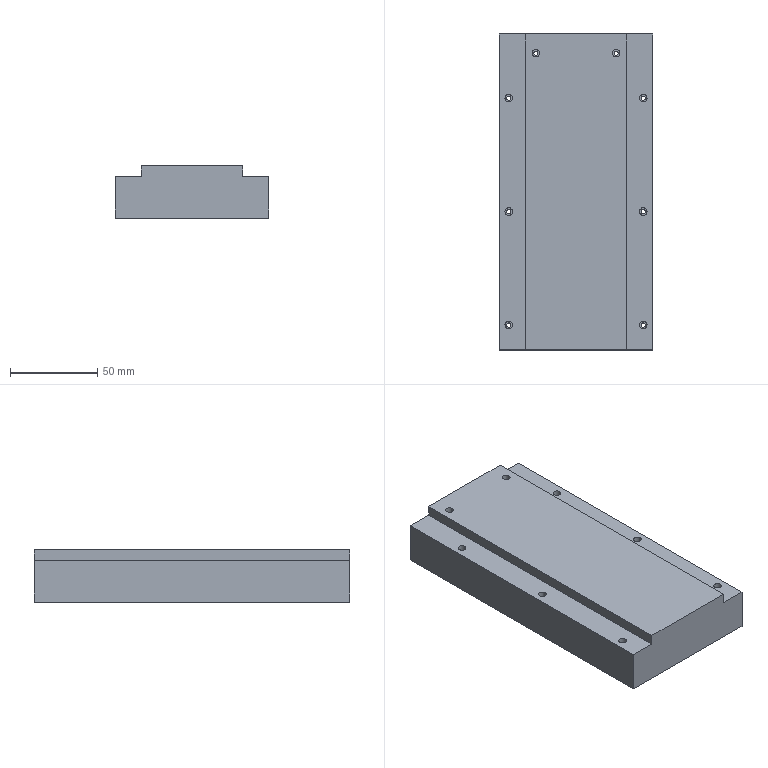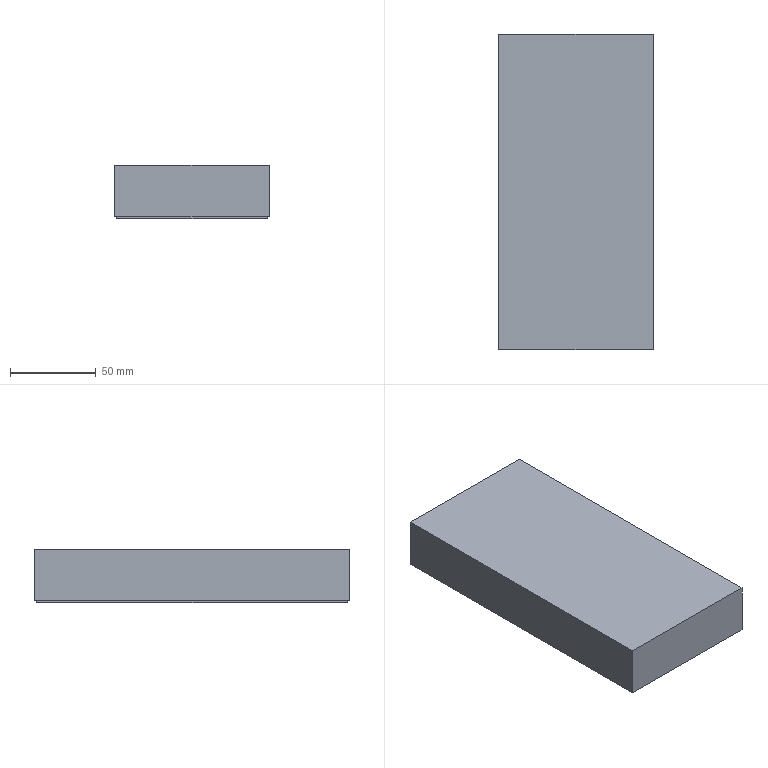CAM job | NX | 3+2 milling, drilling | part box 88 x 181.05 x 30 mm | stock box 90 x 184 x 31 mm
Tools:
number,name,description,diameter,corner_radius,flute_length,length,flutes
0,D4.2,Milling Tool-5 Parameters,4.2,0.0,50.0,75.0,2
10,D3-9-D4-50-3T-FINISH,D3-9-D4-50-3T-精,3.0,0.0,9.0,10.0,2
8,D5-15-D6-50-3T-ROUGH,D5-15-D6-50-3T,5.0,0.0,15.0,16.0,3
0,D5-15-D6-50-3T-FINISH,D5-20-D5-75-3T,5.0,0.0,20.0,75.0,3
10,D6-18-D6-50-3T-ROUGH,D6-18-D6-50-3T-粗,6.0,0.0,18.0,50.0,2
9,D6-18-D6-50-3T-FINISH,D6-18-D6-50-3T,6.0,0.0,18.0,50.0,3
2,D12-36-D12-75-3T-ROUGH,D12-36-D12-75-3T,12.0,0.0,36.0,75.0,3
3,D12-36-D12-120-3T-FINISH,D12-55-D12-120-3T,12.0,0.0,55.0,120.0,3
3,D16-48-D16-100-3T-FINISH,D16-48-D16-100-3T,16.0,0.0,48.0,100.0,3
2,D16-48-D16-100-3T-ROUGH,,16.0,0.0,45.0,100.0,2
1,D63_FACE_MILL,D63面刀,63.0,0.0,30.0,30.0,4
12,DRILL_D1.84-11-D3-40,钻刀D1.84-11-D3-40,1.84,0.0,11.0,12.0,2
7,DRILL_D2.4-29-55,钻刀D2.1-29-55,2.4,0.0,29.0,55.0,2
5,DRILL_D4.2-54-83,钻刀D4.2-54-83,4.2,0.0,54.0,83.0,2
13,FORM_TAP_M2-12-D3-39,挤压M2-12-D3-39,2.0,0.0,12.5,14.5,2
4,CHAMFER_D6-90DEG,倒角D6-90度,6.0,0.0,5.0,50.0,2
14,BALL_END_R1-4-D4-50,球刀R1-4-D4-50,3.0,1.5,4.0,4.5,2
Operations:
program,operation,operation_type,tool,method,geometry_group,spindle_rpm,surface_speed,feed_per_tooth,feed_cut,feed_plunge,cut_length_mm,path_length_mm,cut_time_min,machine_time_min
A1,PLANAR_MILL,PlanarMilling,D63_FACE_MILL,METHOD,WORKPIECE_54,4500.0,890.0,0.0556,1000.0,100.0,254.05,310.05,0.2541,0.2597
A1,DYNAMIC_ROUGH,CavityMilling,D16-48-D16-100-3T-ROUGH,METHOD,WORKPIECE_54,5500.0,207.0,0.1818,3000.0,100.0,8391.846,8926.821,2.703,2.757
A1,PLANAR_MILL_1,PlanarMilling,D16-48-D16-100-3T-FINISH,METHOD,WORKPIECE_54,4500.0,169.0,0.0741,1000.0,100.0,876.2,1646.892,0.8762,0.9533
A1,PLANAR_MILL_1_COPY,PlanarMilling,D16-48-D16-100-3T-FINISH,METHOD,WORKPIECE_54,4500.0,169.0,0.0741,1000.0,100.0,609.512,717.512,0.6095,0.6203
A1,DRILLING,Operation,CHAMFER_D6-90DEG,METHOD,WORKPIECE_54,3000.0,56.0,0.0333,200.0,0.0,10.4,129.898,0.052,0.0639
A1,DRILLING_COPY,Operation,CHAMFER_D6-90DEG,METHOD,WORKPIECE_54,3000.0,56.0,0.0333,200.0,0.0,31.2,486.735,0.156,0.2016
A1,PLANAR_MILL_2,PlanarMilling,CHAMFER_D6-90DEG,METHOD,WORKPIECE_54,3000.0,56.0,0.1667,1000.0,100.0,502.69,560.69,0.5027,0.5085
A1,DRILLING_1_COPY_1,Operation,DRILL_D4.2-54-83,METHOD,WORKPIECE_54,3000.0,39.0,0.0333,200.0,0.0,57.6,224.298,0.288,0.3047
A1,DRILLING_1_COPY_COPY,Operation,DRILL_D4.2-54-83,METHOD,WORKPIECE_54,3000.0,39.0,0.0333,200.0,0.0,136.8,697.935,0.684,0.7401
A1,DRILLING_1,Operation,DRILL_D2.4-29-55,METHOD,WORKPIECE_54,3000.0,22.0,0.025,150.0,0.0,22.0,203.098,0.1467,0.1648
A1,DRILLING_1_COPY,Operation,DRILL_D2.4-29-55,METHOD,WORKPIECE_54,3000.0,22.0,0.025,150.0,0.0,61.326,584.988,0.4088,0.4612
A1,DRILLING_1_COPY_COPY_COPY,Operation,D4.2,METHOD,WORKPIECE_54,1600.0,21.0,0.0312,100.0,0.0,132.0,688.335,1.32,1.376
A1,DRILLING_1_COPY_1_COPY,Operation,D4.2,METHOD,WORKPIECE_54,1600.0,21.0,0.0312,100.0,0.0,56.0,221.098,0.56,0.5765
B1,DYNAMIC_ROUGH_1,CavityMilling,D12-36-D12-75-3T-ROUGH,METHOD,WORKPIECE_55,6500.0,100.0,0.1282,2500.0,100.0,13433.284,14325.003,5.008,5.097
B1,DYNAMIC_ROUGH_1_COPY_1,CavityMilling,D12-36-D12-75-3T-ROUGH,METHOD,WORKPIECE_55,6500.0,100.0,0.1282,2500.0,100.0,11165.241,11496.305,4.284,4.317
B1,DYNAMIC_ROUGH_1_COPY,CavityMilling,D12-36-D12-75-3T-ROUGH,METHOD,WORKPIECE_55,6500.0,100.0,0.1282,2500.0,100.0,4524.864,4559.714,1.787,1.791
B1,PLANAR_MILL_3,PlanarMilling,D63_FACE_MILL,METHOD,WORKPIECE_55,4500.0,890.0,0.0444,800.0,100.0,529.1,563.1,0.6614,0.6648
B1,PLANAR_MILL_4,PlanarMilling,D5-15-D6-50-3T-ROUGH,METHOD,WORKPIECE_55,5000.0,78.0,0.1,1500.0,100.0,347.612,626.435,0.2317,0.2596
B1,PLANAR_MILL_4_COPY,PlanarMilling,D5-15-D6-50-3T-ROUGH,METHOD,WORKPIECE_55,5000.0,78.0,0.1,1500.0,100.0,275.145,1577.731,0.1834,0.3137
B1,PLANAR_MILL_4_COPY_COPY,PlanarMilling,D5-15-D6-50-3T-ROUGH,METHOD,WORKPIECE_55,5000.0,78.0,0.1,1500.0,100.0,1650.441,2405.31,1.1,1.176
B1,PLANAR_MILL_6_COPY_1_COPY,PlanarMilling,D5-15-D6-50-3T-ROUGH,METHOD,WORKPIECE_55,5500.0,103.0,0.0606,1000.0,100.0,555.259,594.459,0.5553,0.5592
B1,PLANAR_MILL_8,PlanarMilling,D6-18-D6-50-3T-FINISH,METHOD,WORKPIECE_55,4500.0,84.0,0.0519,700.0,100.0,554.658,600.658,0.7924,0.797
B1,PLANAR_MILL_5,PlanarMilling,D6-18-D6-50-3T-FINISH,METHOD,WORKPIECE_55,4500.0,84.0,0.0519,700.0,100.0,463.837,579.837,0.6626,0.6742
B1,PLANAR_MILL_5_COPY,PlanarMilling,D6-18-D6-50-3T-FINISH,METHOD,WORKPIECE_55,4500.0,84.0,0.0519,700.0,100.0,451.814,497.814,0.6454,0.65
B1,PLANAR_MILL_6,PlanarMilling,D6-18-D6-50-3T-FINISH,METHOD,WORKPIECE_55,4500.0,84.0,0.0519,700.0,100.0,541.141,580.541,0.7731,0.777
B1,PLANAR_MILL_6_COPY_1,PlanarMilling,D6-18-D6-50-3T-FINISH,METHOD,WORKPIECE_55,4500.0,84.0,0.0519,700.0,100.0,284.066,323.466,0.4058,0.4097
B1,PLANAR_MILL_6_COPY,PlanarMilling,D6-18-D6-50-3T-FINISH,METHOD,WORKPIECE_55,4500.0,84.0,0.0519,700.0,100.0,444.991,482.991,0.6357,0.6395
B1,PLANAR_MILL_6_COPY_COPY,PlanarMilling,D6-18-D6-50-3T-FINISH,METHOD,WORKPIECE_55,4500.0,84.0,0.0519,700.0,100.0,93.0,131.0,0.1329,0.1367
B1,PLANAR_MILL_7_COPY,PlanarMilling,D6-18-D6-50-3T-ROUGH,METHOD,WORKPIECE_55,4500.0,84.0,0.0519,700.0,100.0,744.962,830.362,1.064,1.073
B1,DRILLING_2,Operation,CHAMFER_D6-90DEG,METHOD,WORKPIECE_55,3000.0,56.0,0.0417,250.0,0.0,24.0,277.552,0.096,0.1214
B1,DRILLING_3,Operation,CHAMFER_D6-90DEG,METHOD,WORKPIECE_55,3000.0,56.0,0.0417,250.0,0.0,33.6,494.983,0.1344,0.1805
B1,PLANAR_CHAMFER_MILL,PlanarMilling,CHAMFER_D6-90DEG,METHOD,WORKPIECE_55,4500.0,84.0,0.1111,1000.0,100.0,431.428,467.028,0.4314,0.435
B1,PLANAR_CHAMFER_MILL_4,PlanarMilling,CHAMFER_D6-90DEG,METHOD,WORKPIECE_55,4500.0,84.0,0.1111,1000.0,100.0,454.156,494.156,0.4542,0.4582
B1,PLANAR_CHAMFER_MILL_1,PlanarMilling,CHAMFER_D6-90DEG,METHOD,WORKPIECE_55,4500.0,84.0,0.1111,1000.0,100.0,293.069,330.069,0.2931,0.2968
B1,PLANAR_CHAMFER_MILL_3,PlanarMilling,CHAMFER_D6-90DEG,METHOD,WORKPIECE_55,4500.0,84.0,0.1111,1000.0,100.0,260.237,299.637,0.2602,0.2642
B1,PLANAR_CHAMFER_MILL_2,PlanarMilling,CHAMFER_D6-90DEG,METHOD,WORKPIECE_55,4500.0,84.0,0.1111,1000.0,100.0,236.41,272.41,0.2364,0.24
B1,DRILLING_2_COPY,Operation,DRILL_D1.84-11-D3-40,METHOD,WORKPIECE_55,2000.0,11.0,0.0375,150.0,0.0,42.0,313.552,0.28,0.3072
B1,DRILLING_2_COPY_COPY,Operation,FORM_TAP_M2-12-D3-39,METHOD,WORKPIECE_55,200.0,1.0,0.0007,80.0,0.0,36.0,301.552,0.45,0.4766
C1,DYNAMIC_ROUGH_2,CavityMilling,D5-15-D6-50-3T-ROUGH,METHOD,WORKPIECE_56,6500.0,100.0,0.1178,3000.0,100.0,5406.099,5517.798,1.785,1.796
C1,LOW_WALL_ROUGH_FACE,VolumeBased25DMillingOperation,D6-18-D6-50-3T-FINISH,METHOD,WORKPIECE_56,4500.0,84.0,0.0444,600.0,100.0,471.547,595.343,0.7859,0.7983
C1,LOW_WALL_ROUGH_FACE_COPY,VolumeBased25DMillingOperation,D6-18-D6-50-3T-FINISH,METHOD,WORKPIECE_56,4500.0,84.0,0.0444,600.0,100.0,166.548,289.144,0.2776,0.2898
3-2,DYNAMIC_ROUGH_3_COPY_1,CavityMilling,D12-36-D12-75-3T-ROUGH,METHOD,W3-2,6500.0,100.0,0.1178,3000.0,100.0,25487.224,29483.847,7.442,7.841
3-2,PLANAR_MILL_10_COPY_COPY,PlanarMilling,D12-36-D12-75-3T-ROUGH,METHOD,3-2,6500.0,245.0,0.041,800.0,100.0,640.678,694.678,0.8008,0.8062
3-2,FLOOR_WALL_COPY_1,VolumeBased25DMillingOperation,D12-36-D12-75-3T-ROUGH,METHOD,3-2,6500.0,245.0,0.041,800.0,100.0,457.832,517.732,0.5723,0.5783
3-2,PLANAR_MILL_9_COPY_COPY_COPY,PlanarMilling,D12-36-D12-75-3T-ROUGH,METHOD,3-2,6500.0,245.0,0.041,800.0,100.0,113.299,167.299,0.1416,0.147
3-2,FLOOR_WALL_2_COPY_COPY,VolumeBased25DMillingOperation,D12-36-D12-75-3T-ROUGH,METHOD,3-2,6500.0,245.0,0.041,800.0,100.0,644.283,704.183,0.8054,0.8113
3-2,PLANAR_MILL_12_COPY_1,PlanarMilling,D12-36-D12-75-3T-ROUGH,METHOD,3-2,6500.0,245.0,0.041,800.0,100.0,223.63,437.69,0.2795,0.3009
3-2,FLOOR_WALL_2_COPY_1_COPY_1,VolumeBased25DMillingOperation,D12-36-D12-75-3T-ROUGH,METHOD,3-2,6500.0,245.0,0.041,800.0,100.0,623.096,682.996,0.7789,0.7849
3-2,PLANAR_MILL_9_COPY_1_COPY,PlanarMilling,D12-36-D12-120-3T-FINISH,METHOD,3-2,4500.0,169.0,0.0593,800.0,100.0,113.299,167.299,0.1416,0.147
3-2,PLANAR_MILL_10_COPY_1,PlanarMilling,D12-36-D12-120-3T-FINISH,METHOD,3-2,4500.0,169.0,0.0593,800.0,100.0,640.678,694.678,0.8008,0.8062
3-2,PLANAR_MILL_13_COPY,PlanarMilling,D12-36-D12-120-3T-FINISH,METHOD,3-2,4500.0,169.0,0.0593,800.0,100.0,103.299,159.299,0.1291,0.1347
3-2,FLOOR_WALL_COPY_COPY,VolumeBased25DMillingOperation,D12-36-D12-120-3T-FINISH,METHOD,3-2,4500.0,169.0,0.0593,800.0,100.0,457.832,517.832,0.5723,0.5783
3-2,PLANAR_MILL_12_COPY_COPY,PlanarMilling,D12-36-D12-120-3T-FINISH,METHOD,3-2,4500.0,169.0,0.0593,800.0,100.0,223.63,437.69,0.2795,0.3009
3-2,FLOOR_WALL_2_COPY_2,VolumeBased25DMillingOperation,D12-36-D12-120-3T-FINISH,METHOD,3-2,4500.0,169.0,0.0593,800.0,100.0,644.283,704.183,0.8054,0.8113
3-2,FLOOR_WALL_2_COPY_1_COPY_COPY,VolumeBased25DMillingOperation,D12-36-D12-120-3T-FINISH,METHOD,3-2,4500.0,169.0,0.0593,800.0,100.0,623.096,683.096,0.7789,0.7849
3-2,CURVE_DRIVE_3_COPY,SurfaceContour,BALL_END_R1-4-D4-50,METHOD,3-2,6500.0,40.0,0.1538,2000.0,100.0,7347.416,7533.939,3.674,3.692
3-2,CURVE_DRIVE_COPY,SurfaceContour,BALL_END_R1-4-D4-50,METHOD,3-2,6500.0,40.0,0.1538,2000.0,100.0,2656.034,2656.034,1.328,1.328
D1,DYNAMIC_ROUGH_3,CavityMilling,D12-36-D12-75-3T-ROUGH,METHOD,WORKPIECE_57,6500.0,100.0,0.1178,3000.0,100.0,25487.224,28839.847,7.442,7.777
D2,PLANAR_MILL_9_COPY,PlanarMilling,D12-36-D12-120-3T-FINISH,METHOD,WORKPIECE_57,3500.0,131.0,0.0762,800.0,100.0,113.299,191.199,0.1416,0.1494
D2,PLANAR_MILL_9_COPY_COPY_1,PlanarMilling,D12-36-D12-120-3T-FINISH,METHOD,W3-2,3500.0,131.0,0.0762,800.0,100.0,113.299,211.299,0.1416,0.1514
D-G57,PLANAR_MILL_9,PlanarMilling,D12-36-D12-120-3T-FINISH,METHOD,WORKPIECE_57,3500.0,131.0,0.0762,800.0,100.0,113.299,191.299,0.1416,0.1494
D7,CURVE_DRIVE_1,SurfaceContour,BALL_END_R1-4-D4-50,METHOD,D-G57,6500.0,40.0,0.1538,2000.0,100.0,722.748,757.548,0.3614,0.3649
D7,CURVE_DRIVE_1_COPY,SurfaceContour,BALL_END_R1-4-D4-50,METHOD,D-G57,6500.0,40.0,0.1538,2000.0,100.0,720.168,754.368,0.3601,0.3635
D7,CURVE_DRIVE_1_COPY_1,SurfaceContour,BALL_END_R1-4-D4-50,METHOD,D-G57,6500.0,40.0,0.1538,2000.0,100.0,1028.073,1083.873,0.514,0.5196
D7,CURVE_DRIVE_2,SurfaceContour,BALL_END_R1-4-D4-50,METHOD,D-G57,6500.0,40.0,0.0769,1000.0,100.0,6327.489,6466.395,6.327,6.341
D7,CURVE_DRIVE_1_COPY_3,SurfaceContour,BALL_END_R1-4-D4-50,METHOD,3-2,6500.0,40.0,0.1538,2000.0,100.0,722.948,777.548,0.3615,0.3669
D7,CURVE_DRIVE_1_COPY_COPY_1,SurfaceContour,BALL_END_R1-4-D4-50,METHOD,3-2,6500.0,40.0,0.1538,2000.0,100.0,719.768,774.368,0.3599,0.3653
D7,CURVE_DRIVE_1_COPY_1_COPY_1,SurfaceContour,BALL_END_R1-4-D4-50,METHOD,3-2,6500.0,40.0,0.1538,2000.0,100.0,1027.673,1103.873,0.5138,0.5215
D7,CURVE_DRIVE_2_COPY_1,SurfaceContour,BALL_END_R1-4-D4-50,METHOD,3-2,6500.0,40.0,0.0769,1000.0,100.0,6185.739,6362.302,6.186,6.203
D-G57,PLANAR_MILL_9_COPY_2,PlanarMilling,D12-36-D12-120-3T-FINISH,METHOD,W3-2,3500.0,131.0,0.0762,800.0,100.0,113.299,211.299,0.1416,0.1514
E1,PLANAR_MILL_10_COPY,PlanarMilling,D12-36-D12-75-3T-ROUGH,METHOD,E-G58,3500.0,131.0,0.0762,800.0,100.0,640.677,694.551,0.8008,0.8062
E1,PLANAR_MILL_10,PlanarMilling,D12-36-D12-120-3T-FINISH,METHOD,E-G58,3500.0,131.0,0.0762,800.0,100.0,640.677,694.651,0.8008,0.8062
E1,PLANAR_MILL_13,PlanarMilling,D12-36-D12-120-3T-FINISH,METHOD,E-G58,3500.0,131.0,0.0762,800.0,100.0,103.299,159.299,0.1291,0.1347
E2,CURVE_DRIVE_3,SurfaceContour,BALL_END_R1-4-D4-50,METHOD,E-G58,6500.0,40.0,0.1538,2000.0,100.0,5473.757,5532.164,2.737,2.743
G1,FLOOR_WALL,VolumeBased25DMillingOperation,D12-36-D12-75-3T-ROUGH,METHOD,F-G59,3500.0,131.0,0.0762,800.0,100.0,457.832,557.732,0.5723,0.5823
G1,FLOOR_WALL_COPY,VolumeBased25DMillingOperation,D12-36-D12-120-3T-FINISH,METHOD,F-G59,3500.0,131.0,0.0762,800.0,100.0,457.832,557.832,0.5723,0.5823
G54.1,PLANAR_MILL_12,PlanarMilling,D12-36-D12-120-3T-FINISH,METHOD,G54.1,3500.0,131.0,0.0762,800.0,100.0,223.63,397.49,0.2795,0.2969
G54.1,PLANAR_MILL_12_COPY,PlanarMilling,D12-36-D12-120-3T-FINISH,METHOD,G54.1,3500.0,131.0,0.0762,800.0,100.0,223.63,397.69,0.2795,0.2969
G54.1,CURVE_DRIVE,SurfaceContour,BALL_END_R1-4-D4-50,METHOD,G54.1,6500.0,40.0,0.1538,2000.0,100.0,2656.034,2693.253,1.328,1.332
G54.2,FLOOR_WALL_2,VolumeBased25DMillingOperation,D12-36-D12-120-3T-FINISH,METHOD,G54.2,4500.0,169.0,0.0593,800.0,100.0,644.283,678.183,0.8054,0.8087
G54.2,FLOOR_WALL_2_COPY,VolumeBased25DMillingOperation,D12-36-D12-120-3T-FINISH,METHOD,G54.2,4500.0,169.0,0.0593,800.0,100.0,644.283,678.183,0.8054,0.8087
G54.3,FLOOR_WALL_2_COPY_1,VolumeBased25DMillingOperation,D12-36-D12-120-3T-FINISH,METHOD,G54.3,4500.0,169.0,0.0593,800.0,100.0,623.096,656.996,0.7789,0.7823
G54.3,FLOOR_WALL_2_COPY_1_COPY,VolumeBased25DMillingOperation,D12-36-D12-120-3T-FINISH,METHOD,G54.3,4500.0,169.0,0.0593,800.0,100.0,623.096,657.096,0.7789,0.7823
DEOXIDATION,PLANAR_MILL_14,PlanarMilling,D3-9-D4-50-3T-FINISH,METHOD,G54.4,4500.0,42.0,0.0667,600.0,100.0,877.572,1500.565,1.463,1.525
DEOXIDATION,PLANAR_MILL_14_COPY,PlanarMilling,D3-9-D4-50-3T-FINISH,METHOD,G54.4,4500.0,42.0,0.0667,600.0,100.0,699.288,943.48,1.165,1.19
DEOXIDATION,PLANAR_MILL_14_COPY_COPY,PlanarMilling,D3-9-D4-50-3T-FINISH,METHOD,G54.4,4500.0,42.0,0.0667,600.0,100.0,164.283,467.789,0.2738,0.3042
FIXTURE_1,FLOOR_WALL_1,VolumeBased25DMillingOperation,D12-36-D12-75-3T-ROUGH,METHOD,GZ1,4500.0,169.0,0.1111,1500.0,100.0,1751.176,1784.076,1.167,1.171
FIXTURE_1,FLOOR_WALL_1_COPY,VolumeBased25DMillingOperation,D12-36-D12-120-3T-FINISH,METHOD,GZ1,3500.0,131.0,0.0762,800.0,100.0,1752.582,1785.582,2.191,2.194
FIXTURE_1,PLANAR_MILL_11_COPY,PlanarMilling,D12-36-D12-120-3T-FINISH,METHOD,GZ1,3500.0,65.0,0.0762,800.0,100.0,471.024,509.024,0.5888,0.5926
FIXTURE_1,PLANAR_MILL_11,PlanarMilling,D5-15-D6-50-3T-FINISH,METHOD,GZ1,3500.0,65.0,0.0762,800.0,100.0,510.435,548.435,0.638,0.6418
FIXTURE_1,DRILLING_4,Operation,CHAMFER_D6-90DEG,METHOD,GZ1,2000.0,37.0,0.05,200.0,0.0,32.0,540.637,0.16,0.2109
FIXTURE_1,DRILLING_5,Operation,DRILL_D1.84-11-D3-40,METHOD,GZ1,2500.0,14.0,0.03,150.0,0.0,144.0,764.637,0.96,1.022
FIXTURE_1,DRILLING_5_COPY,Operation,FORM_TAP_M2-12-D3-39,METHOD,GZ1,300.0,1.0,0.2,120.0,0.0,72.0,620.637,0.6,0.6549